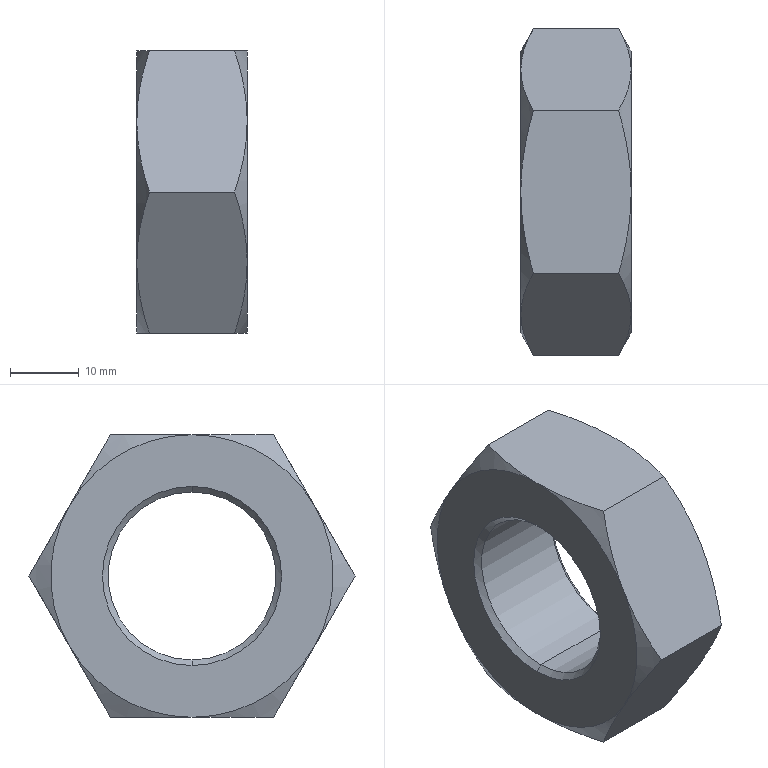Part | STEP file | NT-10(CQ2)_HI | 1 solid | 26 faces | box 16 x 47.343 x 41 mm | volume 15625 mm3 | cone 16 | plane 8 | cylinder 2 | commonest cylinder face diameters 24.376 x2